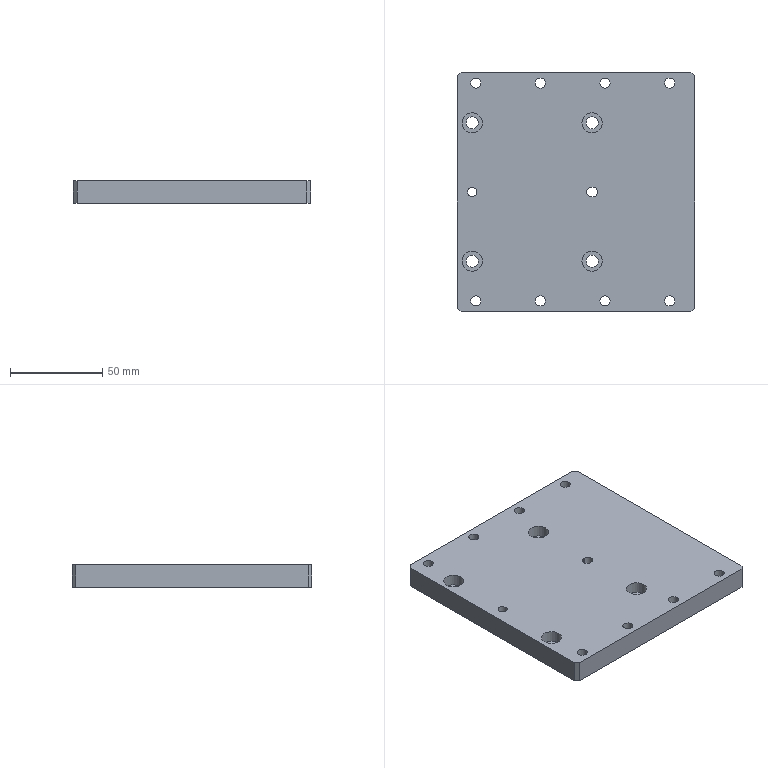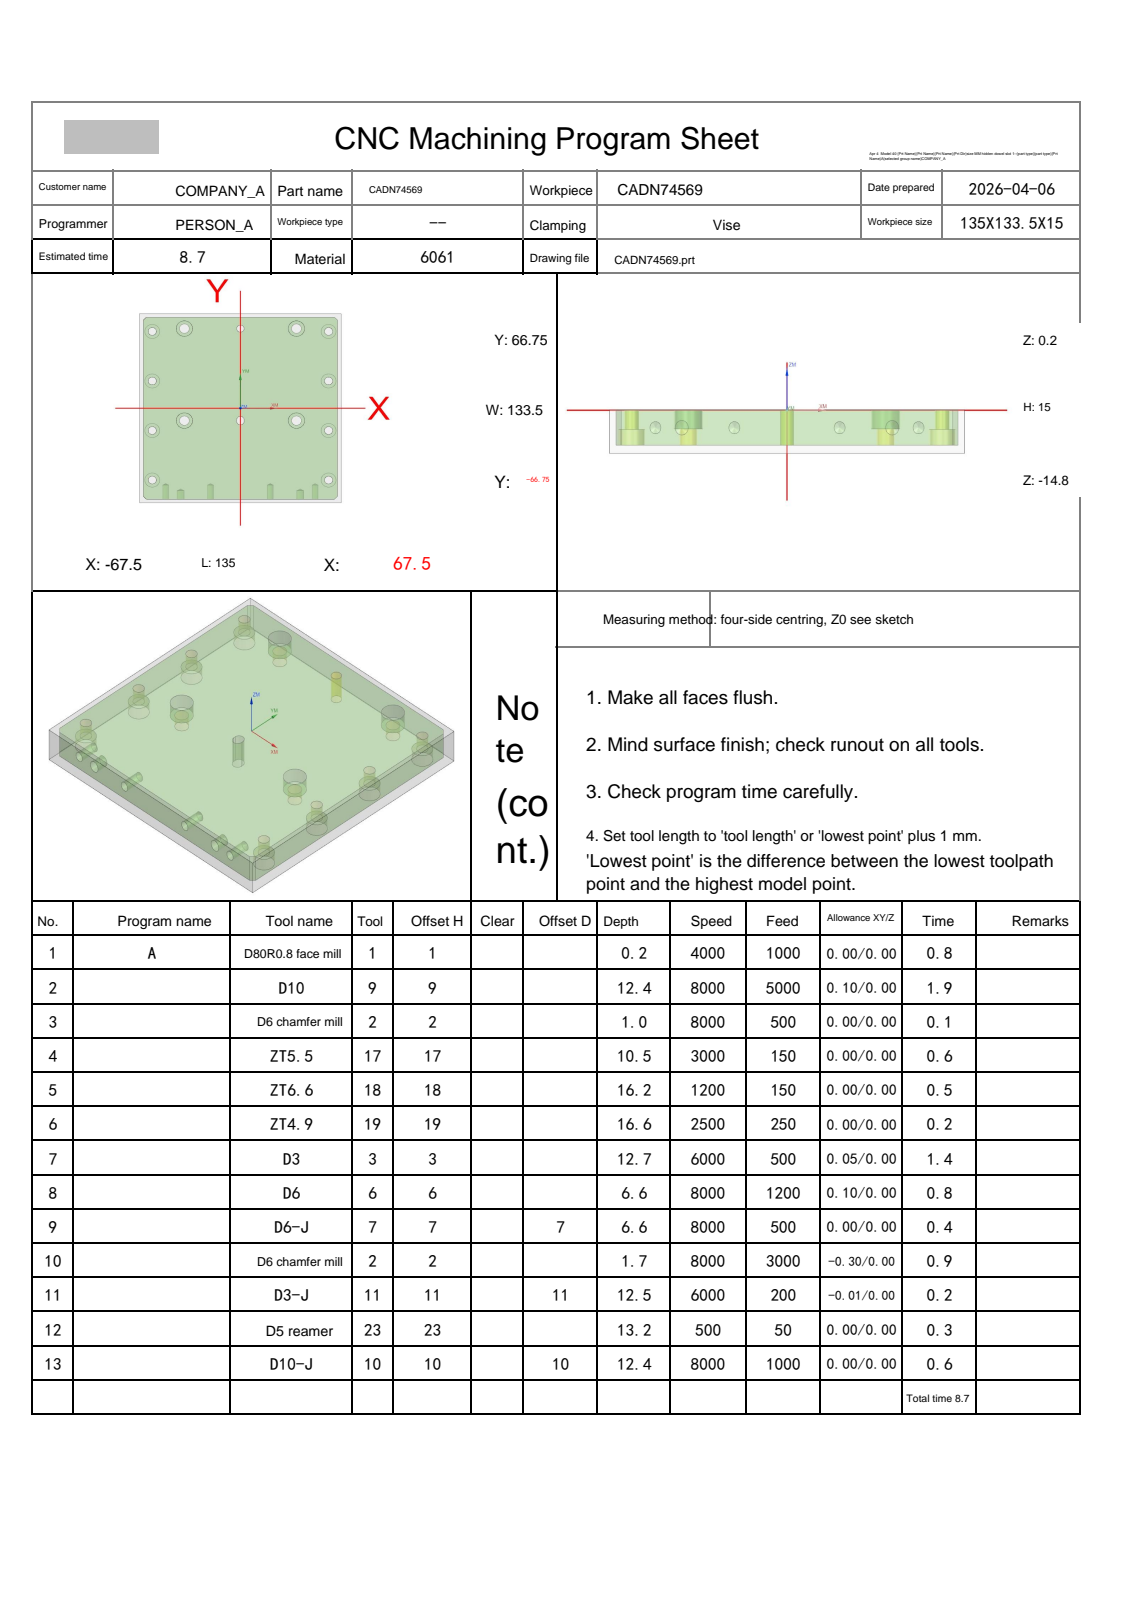NC program | NX | posted by the shop | part box 128.5 x 130 x 12 mm
Whole program, first 1332 of 1585 lines:
%
O0001
(Machine time: 11.02 MIN)
(===Total Tool:12===)
(T1=D80R0.8 face mill D=80.  R=0.8  D-  H01 Z=0.    )
(T9=D10     D=10.  R=0.   D-  H09 Z=-12.2 )
(T2=D6 chamfer mill   D=6.   R=0.   D-  H02 Z=-1.5  )
(T17=ZT5.5  D=5.5  DR_a=118 D-  H17 Z=-10.25)
(T18=ZT6.6  D=6.6  DR_a=118 D-  H18 Z=-15.98)
(T19=ZT4.9  D=4.9  DR_a=120 D-  H19 Z=-16.41)
(T3=D3      D=3.   R=0.   D-  H03 Z=-12.5 )
(T6=D6      D=6.   R=0.   D-  H06 Z=-6.4  )
(T7=D6-J    D=6.   R=0.   D7  H07 Z=-6.4  )
(T11=D3-J   D=3.   R=0.   D11 H11 Z=-12.3 )
(T23=D5 reamer   D=5.   DR_a=180 D-  H23 Z=-13.  )
(T10=D10-J  D=10.  R=0.   D10 H10 Z=-12.2 )
G80 G90 G17 G49 G40
G91 G28 Z0
M01
N1 T01 M06
(D80R0.8 face mill  D=80. R=0.8 H=01 ce=0.00 di=0.00)
G00 G90 G54 X-110. Y52.125 M03 S4000
G43 H01 Z20.
M08
Z2.
G01 Z0.0 F1000.
X-105.
X105.
Y0.0
X-105.
Y-52.125
X105.
X110.
Z2.
G00 Z20.
G91 G28 Z0.0
M05
M09
G91 G28 Z0.0
M01
N2 T09 M06
(D10  D=10. R=0. H=09 ce=0.10 di=0.00)
G00 G90 G54 X0.0 Y69.35 M03 S8000
G43 H09 Z20.
M08
Z.5
G01 X63. Z.408 F5000.
G02 X66.606 Y67.856 Z.402 I0.0 J-5.1
G01 X68.606 Y65.856 Z.398
G02 X70.1 Y62.25 Z.392 I-3.606 J-3.606
G01 Y-62.25 Z.211
G02 X68.606 Y-65.856 Z.205 I-5.1 J0.0
G01 X66.606 Y-67.856 Z.201
G02 X63. Y-69.35 Z.195 I-3.606 J3.606
G01 X-63. Z.011
G02 X-66.606 Y-67.856 Z.005 I0.0 J5.1
G01 X-68.606 Y-65.856 Z.001
G02 X-70.1 Y-62.25 Z-.005 I3.606 J3.606
G01 Y62.25 Z-.186
G02 X-68.606 Y65.856 Z-.192 I5.1 J0.0
G01 X-66.606 Y67.856 Z-.196
G02 X-63. Y69.35 Z-.202 I3.606 J-3.606
G01 X63. Z-.386
G02 X66.606 Y67.856 Z-.391 I0.0 J-5.1
G01 X68.606 Y65.856 Z-.396
G02 X70.1 Y62.25 Z-.401 I-3.606 J-3.606
G01 Y-62.25 Z-.583
G02 X68.606 Y-65.856 Z-.589 I-5.1 J0.0
G01 X66.606 Y-67.856 Z-.593
G02 X63. Y-69.35 Z-.599 I-3.606 J3.606
G01 X-63. Z-.782
G02 X-66.606 Y-67.856 Z-.788 I0.0 J5.1
G01 X-68.606 Y-65.856 Z-.792
G02 X-70.1 Y-62.25 Z-.798 I3.606 J3.606
G01 Y62.25 Z-.98
G02 X-68.606 Y65.856 Z-.986 I5.1 J0.0
G01 X-66.606 Y67.856 Z-.99
G02 X-63. Y69.35 Z-.996 I3.606 J-3.606
G01 X63. Z-1.179
G02 X66.606 Y67.856 Z-1.185 I0.0 J-5.1
G01 X68.606 Y65.856 Z-1.189
G02 X70.1 Y62.25 Z-1.195 I-3.606 J-3.606
G01 Y-62.25 Z-1.377
G02 X68.606 Y-65.856 Z-1.383 I-5.1 J0.0
G01 X66.606 Y-67.856 Z-1.387
G02 X63. Y-69.35 Z-1.393 I-3.606 J3.606
G01 X-63. Z-1.576
G02 X-66.606 Y-67.856 Z-1.582 I0.0 J5.1
G01 X-68.606 Y-65.856 Z-1.586
G02 X-70.1 Y-62.25 Z-1.592 I3.606 J3.606
G01 Y62.25 Z-1.774
G02 X-68.606 Y65.856 Z-1.779 I5.1 J0.0
G01 X-66.606 Y67.856 Z-1.784
G02 X-63. Y69.35 Z-1.789 I3.606 J-3.606
G01 X63. Z-1.973
G02 X66.606 Y67.856 Z-1.979 I0.0 J-5.1
G01 X68.606 Y65.856 Z-1.983
G02 X70.1 Y62.25 Z-1.989 I-3.606 J-3.606
G01 Y-62.25 Z-2.17
G02 X68.606 Y-65.856 Z-2.176 I-5.1 J0.0
G01 X66.606 Y-67.856 Z-2.18
G02 X63. Y-69.35 Z-2.186 I-3.606 J3.606
G01 X-63. Z-2.37
G02 X-66.606 Y-67.856 Z-2.376 I0.0 J5.1
G01 X-68.606 Y-65.856 Z-2.38
G02 X-70.1 Y-62.25 Z-2.386 I3.606 J3.606
G01 Y62.25 Z-2.567
G02 X-68.606 Y65.856 Z-2.573 I5.1 J0.0
G01 X-66.606 Y67.856 Z-2.577
G02 X-63. Y69.35 Z-2.583 I3.606 J-3.606
G01 X63. Z-2.767
G02 X66.606 Y67.856 Z-2.773 I0.0 J-5.1
G01 X68.606 Y65.856 Z-2.777
G02 X70.1 Y62.25 Z-2.783 I-3.606 J-3.606
G01 Y-62.25 Z-2.964
G02 X68.606 Y-65.856 Z-2.97 I-5.1 J0.0
G01 X66.606 Y-67.856 Z-2.974
G02 X63. Y-69.35 Z-2.98 I-3.606 J3.606
G01 X-63. Z-3.164
G02 X-66.606 Y-67.856 Z-3.17 I0.0 J5.1
G01 X-68.606 Y-65.856 Z-3.174
G02 X-70.1 Y-62.25 Z-3.18 I3.606 J3.606
G01 Y62.25 Z-3.361
G02 X-68.606 Y65.856 Z-3.367 I5.1 J0.0
G01 X-66.606 Y67.856 Z-3.371
G02 X-63. Y69.35 Z-3.377 I3.606 J-3.606
G01 X63. Z-3.561
G02 X66.606 Y67.856 Z-3.566 I0.0 J-5.1
G01 X68.606 Y65.856 Z-3.571
G02 X70.1 Y62.25 Z-3.576 I-3.606 J-3.606
G01 Y-62.25 Z-3.758
G02 X68.606 Y-65.856 Z-3.764 I-5.1 J0.0
G01 X66.606 Y-67.856 Z-3.768
G02 X63. Y-69.35 Z-3.774 I-3.606 J3.606
G01 X-63. Z-3.957
G02 X-66.606 Y-67.856 Z-3.963 I0.0 J5.1
G01 X-68.606 Y-65.856 Z-3.967
G02 X-70.1 Y-62.25 Z-3.973 I3.606 J3.606
G01 Y62.25 Z-4.155
G02 X-68.606 Y65.856 Z-4.161 I5.1 J0.0
G01 X-66.606 Y67.856 Z-4.165
G02 X-63. Y69.35 Z-4.171 I3.606 J-3.606
G01 X63. Z-4.354
G02 X66.606 Y67.856 Z-4.36 I0.0 J-5.1
G01 X68.606 Y65.856 Z-4.364
G02 X70.1 Y62.25 Z-4.37 I-3.606 J-3.606
G01 Y-62.25 Z-4.552
G02 X68.606 Y-65.856 Z-4.558 I-5.1 J0.0
G01 X66.606 Y-67.856 Z-4.562
G02 X63. Y-69.35 Z-4.568 I-3.606 J3.606
G01 X-63. Z-4.751
G02 X-66.606 Y-67.856 Z-4.757 I0.0 J5.1
G01 X-68.606 Y-65.856 Z-4.761
G02 X-70.1 Y-62.25 Z-4.767 I3.606 J3.606
G01 Y62.25 Z-4.949
G02 X-68.606 Y65.856 Z-4.954 I5.1 J0.0
G01 X-66.606 Y67.856 Z-4.959
G02 X-63. Y69.35 Z-4.964 I3.606 J-3.606
G01 X63. Z-5.148
G02 X66.606 Y67.856 Z-5.154 I0.0 J-5.1
G01 X68.606 Y65.856 Z-5.158
G02 X70.1 Y62.25 Z-5.164 I-3.606 J-3.606
G01 Y-62.25 Z-5.345
G02 X68.606 Y-65.856 Z-5.351 I-5.1 J0.0
G01 X66.606 Y-67.856 Z-5.355
G02 X63. Y-69.35 Z-5.361 I-3.606 J3.606
G01 X-63. Z-5.545
G02 X-66.606 Y-67.856 Z-5.551 I0.0 J5.1
G01 X-68.606 Y-65.856 Z-5.555
G02 X-70.1 Y-62.25 Z-5.561 I3.606 J3.606
G01 Y62.25 Z-5.742
G02 X-68.606 Y65.856 Z-5.748 I5.1 J0.0
G01 X-66.606 Y67.856 Z-5.752
G02 X-63. Y69.35 Z-5.758 I3.606 J-3.606
G01 X63. Z-5.942
G02 X66.606 Y67.856 Z-5.948 I0.0 J-5.1
G01 X68.606 Y65.856 Z-5.952
G02 X70.1 Y62.25 Z-5.958 I-3.606 J-3.606
G01 Y-62.25 Z-6.139
G02 X68.606 Y-65.856 Z-6.145 I-5.1 J0.0
G01 X66.606 Y-67.856 Z-6.149
G02 X63. Y-69.35 Z-6.155 I-3.606 J3.606
G01 X-63. Z-6.339
G02 X-66.606 Y-67.856 Z-6.345 I0.0 J5.1
G01 X-68.606 Y-65.856 Z-6.349
G02 X-70.1 Y-62.25 Z-6.355 I3.606 J3.606
G01 Y62.25 Z-6.536
G02 X-68.606 Y65.856 Z-6.542 I5.1 J0.0
G01 X-66.606 Y67.856 Z-6.546
G02 X-63. Y69.35 Z-6.552 I3.606 J-3.606
G01 X63. Z-6.736
G02 X66.606 Y67.856 Z-6.741 I0.0 J-5.1
G01 X68.606 Y65.856 Z-6.746
G02 X70.1 Y62.25 Z-6.751 I-3.606 J-3.606
G01 Y-62.25 Z-6.933
G02 X68.606 Y-65.856 Z-6.939 I-5.1 J0.0
G01 X66.606 Y-67.856 Z-6.943
G02 X63. Y-69.35 Z-6.949 I-3.606 J3.606
G01 X-63. Z-7.132
G02 X-66.606 Y-67.856 Z-7.138 I0.0 J5.1
G01 X-68.606 Y-65.856 Z-7.142
G02 X-70.1 Y-62.25 Z-7.148 I3.606 J3.606
G01 Y62.25 Z-7.33
G02 X-68.606 Y65.856 Z-7.336 I5.1 J0.0
G01 X-66.606 Y67.856 Z-7.34
G02 X-63. Y69.35 Z-7.346 I3.606 J-3.606
G01 X63. Z-7.529
G02 X66.606 Y67.856 Z-7.535 I0.0 J-5.1
G01 X68.606 Y65.856 Z-7.539
G02 X70.1 Y62.25 Z-7.545 I-3.606 J-3.606
G01 Y-62.25 Z-7.727
G02 X68.606 Y-65.856 Z-7.733 I-5.1 J0.0
G01 X66.606 Y-67.856 Z-7.737
G02 X63. Y-69.35 Z-7.743 I-3.606 J3.606
G01 X-63. Z-7.926
G02 X-66.606 Y-67.856 Z-7.932 I0.0 J5.1
G01 X-68.606 Y-65.856 Z-7.936
G02 X-70.1 Y-62.25 Z-7.942 I3.606 J3.606
G01 Y62.25 Z-8.124
G02 X-68.606 Y65.856 Z-8.129 I5.1 J0.0
G01 X-66.606 Y67.856 Z-8.134
G02 X-63. Y69.35 Z-8.139 I3.606 J-3.606
G01 X63. Z-8.323
G02 X66.606 Y67.856 Z-8.329 I0.0 J-5.1
G01 X68.606 Y65.856 Z-8.333
G02 X70.1 Y62.25 Z-8.339 I-3.606 J-3.606
G01 Y-62.25 Z-8.52
G02 X68.606 Y-65.856 Z-8.526 I-5.1 J0.0
G01 X66.606 Y-67.856 Z-8.53
G02 X63. Y-69.35 Z-8.536 I-3.606 J3.606
G01 X-63. Z-8.72
G02 X-66.606 Y-67.856 Z-8.726 I0.0 J5.1
G01 X-68.606 Y-65.856 Z-8.73
G02 X-70.1 Y-62.25 Z-8.736 I3.606 J3.606
G01 Y62.25 Z-8.917
G02 X-68.606 Y65.856 Z-8.923 I5.1 J0.0
G01 X-66.606 Y67.856 Z-8.927
G02 X-63. Y69.35 Z-8.933 I3.606 J-3.606
G01 X63. Z-9.117
G02 X66.606 Y67.856 Z-9.123 I0.0 J-5.1
G01 X68.606 Y65.856 Z-9.127
G02 X70.1 Y62.25 Z-9.133 I-3.606 J-3.606
G01 Y-62.25 Z-9.314
G02 X68.606 Y-65.856 Z-9.32 I-5.1 J0.0
G01 X66.606 Y-67.856 Z-9.324
G02 X63. Y-69.35 Z-9.33 I-3.606 J3.606
G01 X-63. Z-9.514
G02 X-66.606 Y-67.856 Z-9.52 I0.0 J5.1
G01 X-68.606 Y-65.856 Z-9.524
G02 X-70.1 Y-62.25 Z-9.53 I3.606 J3.606
G01 Y62.25 Z-9.711
G02 X-68.606 Y65.856 Z-9.717 I5.1 J0.0
G01 X-66.606 Y67.856 Z-9.721
G02 X-63. Y69.35 Z-9.727 I3.606 J-3.606
G01 X63. Z-9.911
G02 X66.606 Y67.856 Z-9.916 I0.0 J-5.1
G01 X68.606 Y65.856 Z-9.921
G02 X70.1 Y62.25 Z-9.926 I-3.606 J-3.606
G01 Y-62.25 Z-10.108
G02 X68.606 Y-65.856 Z-10.114 I-5.1 J0.0
G01 X66.606 Y-67.856 Z-10.118
G02 X63. Y-69.35 Z-10.124 I-3.606 J3.606
G01 X-63. Z-10.307
G02 X-66.606 Y-67.856 Z-10.313 I0.0 J5.1
G01 X-68.606 Y-65.856 Z-10.317
G02 X-70.1 Y-62.25 Z-10.323 I3.606 J3.606
G01 Y62.25 Z-10.505
G02 X-68.606 Y65.856 Z-10.511 I5.1 J0.0
G01 X-66.606 Y67.856 Z-10.515
G02 X-63. Y69.35 Z-10.521 I3.606 J-3.606
G01 X63. Z-10.704
G02 X66.606 Y67.856 Z-10.71 I0.0 J-5.1
G01 X68.606 Y65.856 Z-10.714
G02 X70.1 Y62.25 Z-10.72 I-3.606 J-3.606
G01 Y-62.25 Z-10.902
G02 X68.606 Y-65.856 Z-10.908 I-5.1 J0.0
G01 X66.606 Y-67.856 Z-10.912
G02 X63. Y-69.35 Z-10.918 I-3.606 J3.606
G01 X-63. Z-11.101
G02 X-66.606 Y-67.856 Z-11.107 I0.0 J5.1
G01 X-68.606 Y-65.856 Z-11.111
G02 X-70.1 Y-62.25 Z-11.117 I3.606 J3.606
G01 Y62.25 Z-11.299
G02 X-68.606 Y65.856 Z-11.304 I5.1 J0.0
G01 X-66.606 Y67.856 Z-11.309
G02 X-63. Y69.35 Z-11.314 I3.606 J-3.606
G01 X63. Z-11.498
G02 X66.606 Y67.856 Z-11.504 I0.0 J-5.1
G01 X68.606 Y65.856 Z-11.508
G02 X70.1 Y62.25 Z-11.514 I-3.606 J-3.606
G01 Y-62.25 Z-11.695
G02 X68.606 Y-65.856 Z-11.701 I-5.1 J0.0
G01 X66.606 Y-67.856 Z-11.705
G02 X63. Y-69.35 Z-11.711 I-3.606 J3.606
G01 X-63. Z-11.895
G02 X-66.606 Y-67.856 Z-11.901 I0.0 J5.1
G01 X-68.606 Y-65.856 Z-11.905
G02 X-70.1 Y-62.25 Z-11.911 I3.606 J3.606
G01 Y62.25 Z-12.092
G02 X-68.606 Y65.856 Z-12.098 I5.1 J0.0
G01 X-66.606 Y67.856 Z-12.102
G02 X-63. Y69.35 Z-12.108 I3.606 J-3.606
G01 X0.0 Z-12.2
X63.
G02 X66.606 Y67.856 I0.0 J-5.1
G01 X68.606 Y65.856
G02 X70.1 Y62.25 I-3.606 J-3.606
G01 Y-62.25
G02 X68.606 Y-65.856 I-5.1 J0.0
G01 X66.606 Y-67.856
G02 X63. Y-69.35 I-3.606 J3.606
G01 X-63.
G02 X-66.606 Y-67.856 I0.0 J5.1
G01 X-68.606 Y-65.856
G02 X-70.1 Y-62.25 I3.606 J3.606
G01 Y62.25
G02 X-68.606 Y65.856 I5.1 J0.0
G01 X-66.606 Y67.856
G02 X-63. Y69.35 I3.606 J-3.606
G01 X0.0
X.5
Z-11.2
G00 Z20.
G91 G28 Z0.0
M05
M09
G91 G28 Z0.0
M01
N3 T02 M06
(D6 chamfer mill  D=6. R=0. H=02 ce=0.00 di=0.00)
G00 G90 G54 X59. Y-50.75 M03 S8000
G43 H02 Z20.
M08
G98 G81 X59. Y-50.75 Z-.8 R1. F500.
Y-15.75
X37.5 Y-8.75
X59. Y19.25
Y54.25
X37.5 Y56.25
X0.0
X-37.5
X-59. Y54.25
Y19.25
X-37.5 Y-8.75
X-59. Y-15.75
Y-50.75
X0.0 Y-8.25
G80
G00 Z20.
G91 G28 Z0.0
M05
M09
G91 G28 Z0.0
M01
N4 T17 M06
(ZT5.5 D=5.5 DR_a=118 H=17)
G00 G90 G54 X59. Y-50.75 M03 S3000
G43 H17 Z20.
M08
G98 G83 X59. Y-50.75 Z-10.252 R1. F150. Q3.
Y-15.75
Y19.25
Y54.25
X-59.
Y19.25
Y-15.75
Y-50.75
G80
G00 Z20.
G91 G28 Z0.0
M05
M09
G91 G28 Z0.0
M01
N5 T18 M06
(ZT6.6 D=6.6 DR_a=118 H=18)
G00 G90 G54 X-37.5 Y-8.75 M03 S1200
G43 H18 Z20.
M08
G98 G83 X-37.5 Y-8.75 Z-15.983 R1. F150. Q2.
Y56.25
X37.5
Y-8.75
G80
G00 Z20.
G91 G28 Z0.0
M05
M09
G91 G28 Z0.0
M01
N6 T19 M06
(ZT4.9 D=4.9 DR_a=120 H=19)
G00 G90 G54 X0.0 Y56.25 M03 S2500
G43 H19 Z20.
M08
G98 G83 X0.0 Y56.25 Z-16.415 R1. F250. Q2.
Y-8.25
G80
G00 Z20.
G91 G28 Z0.0
M05
M09
G91 G28 Z0.0
M01
N7 T03 M06
(D3  D=3. R=0. H=03 ce=0.05 di=0.00)
G00 G90 G54 X.95 Y-8.75 M03 S6000
G43 H03 Z20.
M08
Z.5
G01 Y-8.25 Z.491 F500.
G03 X0.0 Y-7.3 Z.463 I-.95 J0.0
X-.95 Y-8.25 Z.435 I0.0 J-.95
G01 Y-9.25 Z.416
G03 X0.0 Y-10.2 Z.388 I.95 J0.0
X.95 Y-9.25 Z.36 I0.0 J.95
G01 Y-8.25 Z.341
G03 X0.0 Y-7.3 Z.313 I-.95 J0.0
X-.95 Y-8.25 Z.285 I0.0 J-.95
G01 Y-9.25 Z.266
G03 X0.0 Y-10.2 Z.239 I.95 J0.0
X.95 Y-9.25 Z.211 I0.0 J.95
G01 Y-8.25 Z.192
G03 X0.0 Y-7.3 Z.164 I-.95 J0.0
X-.95 Y-8.25 Z.136 I0.0 J-.95
G01 Y-9.25 Z.117
G03 X0.0 Y-10.2 Z.089 I.95 J0.0
X.95 Y-9.25 Z.061 I0.0 J.95
G01 Y-8.25 Z.042
G03 X0.0 Y-7.3 Z.014 I-.95 J0.0
X-.95 Y-8.25 Z-.014 I0.0 J-.95
G01 Y-9.25 Z-.032
G03 X0.0 Y-10.2 Z-.06 I.95 J0.0
X.95 Y-9.25 Z-.088 I0.0 J.95
G01 Y-8.25 Z-.107
G03 X0.0 Y-7.3 Z-.135 I-.95 J0.0
X-.95 Y-8.25 Z-.163 I0.0 J-.95
G01 Y-9.25 Z-.182
G03 X0.0 Y-10.2 Z-.21 I.95 J0.0
X.95 Y-9.25 Z-.238 I0.0 J.95
G01 Y-8.25 Z-.257
G03 X0.0 Y-7.3 Z-.284 I-.95 J0.0
X-.95 Y-8.25 Z-.312 I0.0 J-.95
G01 Y-9.25 Z-.331
G03 X0.0 Y-10.2 Z-.359 I.95 J0.0
X.95 Y-9.25 Z-.387 I0.0 J.95
G01 Y-8.25 Z-.406
G03 X0.0 Y-7.3 Z-.434 I-.95 J0.0
X-.95 Y-8.25 Z-.462 I0.0 J-.95
G01 Y-9.25 Z-.481
G03 X0.0 Y-10.2 Z-.509 I.95 J0.0
X.95 Y-9.25 Z-.537 I0.0 J.95
G01 Y-8.25 Z-.555
G03 X0.0 Y-7.3 Z-.583 I-.95 J0.0
X-.95 Y-8.25 Z-.611 I0.0 J-.95
G01 Y-9.25 Z-.63
G03 X0.0 Y-10.2 Z-.658 I.95 J0.0
X.95 Y-9.25 Z-.686 I0.0 J.95
G01 Y-8.25 Z-.705
G03 X0.0 Y-7.3 Z-.733 I-.95 J0.0
X-.95 Y-8.25 Z-.761 I0.0 J-.95
G01 Y-9.25 Z-.779
G03 X0.0 Y-10.2 Z-.807 I.95 J0.0
X.95 Y-9.25 Z-.835 I0.0 J.95
G01 Y-8.25 Z-.854
G03 X0.0 Y-7.3 Z-.882 I-.95 J0.0
X-.95 Y-8.25 Z-.91 I0.0 J-.95
G01 Y-9.25 Z-.929
G03 X0.0 Y-10.2 Z-.957 I.95 J0.0
X.95 Y-9.25 Z-.985 I0.0 J.95
G01 Y-8.25 Z-1.004
G03 X0.0 Y-7.3 Z-1.032 I-.95 J0.0
X-.95 Y-8.25 Z-1.06 I0.0 J-.95
G01 Y-9.25 Z-1.078
G03 X0.0 Y-10.2 Z-1.106 I.95 J0.0
X.95 Y-9.25 Z-1.134 I0.0 J.95
G01 Y-8.25 Z-1.153
G03 X0.0 Y-7.3 Z-1.181 I-.95 J0.0
X-.95 Y-8.25 Z-1.209 I0.0 J-.95
G01 Y-9.25 Z-1.228
G03 X0.0 Y-10.2 Z-1.256 I.95 J0.0
X.95 Y-9.25 Z-1.284 I0.0 J.95
G01 Y-8.25 Z-1.302
G03 X0.0 Y-7.3 Z-1.33 I-.95 J0.0
X-.95 Y-8.25 Z-1.358 I0.0 J-.95
G01 Y-9.25 Z-1.377
G03 X0.0 Y-10.2 Z-1.405 I.95 J0.0
X.95 Y-9.25 Z-1.433 I0.0 J.95
G01 Y-8.25 Z-1.452
G03 X0.0 Y-7.3 Z-1.48 I-.95 J0.0
X-.95 Y-8.25 Z-1.508 I0.0 J-.95
G01 Y-9.25 Z-1.527
G03 X0.0 Y-10.2 Z-1.555 I.95 J0.0
X.95 Y-9.25 Z-1.583 I0.0 J.95
G01 Y-8.25 Z-1.601
G03 X0.0 Y-7.3 Z-1.629 I-.95 J0.0
X-.95 Y-8.25 Z-1.657 I0.0 J-.95
G01 Y-9.25 Z-1.676
G03 X0.0 Y-10.2 Z-1.704 I.95 J0.0
X.95 Y-9.25 Z-1.732 I0.0 J.95
G01 Y-8.25 Z-1.751
G03 X0.0 Y-7.3 Z-1.779 I-.95 J0.0
X-.95 Y-8.25 Z-1.807 I0.0 J-.95
G01 Y-9.25 Z-1.825
G03 X0.0 Y-10.2 Z-1.853 I.95 J0.0
X.95 Y-9.25 Z-1.881 I0.0 J.95
G01 Y-8.25 Z-1.9
G03 X0.0 Y-7.3 Z-1.928 I-.95 J0.0
X-.95 Y-8.25 Z-1.956 I0.0 J-.95
G01 Y-9.25 Z-1.975
G03 X0.0 Y-10.2 Z-2.003 I.95 J0.0
X.95 Y-9.25 Z-2.031 I0.0 J.95
G01 Y-8.25 Z-2.05
G03 X0.0 Y-7.3 Z-2.078 I-.95 J0.0
X-.95 Y-8.25 Z-2.106 I0.0 J-.95
G01 Y-9.25 Z-2.124
G03 X0.0 Y-10.2 Z-2.152 I.95 J0.0
X.95 Y-9.25 Z-2.18 I0.0 J.95
G01 Y-8.25 Z-2.199
G03 X0.0 Y-7.3 Z-2.227 I-.95 J0.0
X-.95 Y-8.25 Z-2.255 I0.0 J-.95
G01 Y-9.25 Z-2.274
G03 X0.0 Y-10.2 Z-2.302 I.95 J0.0
X.95 Y-9.25 Z-2.33 I0.0 J.95
G01 Y-8.25 Z-2.348
G03 X0.0 Y-7.3 Z-2.376 I-.95 J0.0
X-.95 Y-8.25 Z-2.404 I0.0 J-.95
G01 Y-9.25 Z-2.423
G03 X0.0 Y-10.2 Z-2.451 I.95 J0.0
X.95 Y-9.25 Z-2.479 I0.0 J.95
G01 Y-8.25 Z-2.498
G03 X0.0 Y-7.3 Z-2.526 I-.95 J0.0
X-.95 Y-8.25 Z-2.554 I0.0 J-.95
G01 Y-9.25 Z-2.573
G03 X0.0 Y-10.2 Z-2.601 I.95 J0.0
X.95 Y-9.25 Z-2.629 I0.0 J.95
G01 Y-8.25 Z-2.647
G03 X0.0 Y-7.3 Z-2.675 I-.95 J0.0
X-.95 Y-8.25 Z-2.703 I0.0 J-.95
G01 Y-9.25 Z-2.722
G03 X0.0 Y-10.2 Z-2.75 I.95 J0.0
X.95 Y-9.25 Z-2.778 I0.0 J.95
G01 Y-8.25 Z-2.797
G03 X0.0 Y-7.3 Z-2.825 I-.95 J0.0
X-.95 Y-8.25 Z-2.853 I0.0 J-.95
G01 Y-9.25 Z-2.871
G03 X0.0 Y-10.2 Z-2.899 I.95 J0.0
X.95 Y-9.25 Z-2.927 I0.0 J.95
G01 Y-8.25 Z-2.946
G03 X0.0 Y-7.3 Z-2.974 I-.95 J0.0
X-.95 Y-8.25 Z-3.002 I0.0 J-.95
G01 Y-9.25 Z-3.021
G03 X0.0 Y-10.2 Z-3.049 I.95 J0.0
X.95 Y-9.25 Z-3.077 I0.0 J.95
G01 Y-8.25 Z-3.096
G03 X0.0 Y-7.3 Z-3.124 I-.95 J0.0
X-.95 Y-8.25 Z-3.152 I0.0 J-.95
G01 Y-9.25 Z-3.17
G03 X0.0 Y-10.2 Z-3.198 I.95 J0.0
X.95 Y-9.25 Z-3.226 I0.0 J.95
G01 Y-8.25 Z-3.245
G03 X0.0 Y-7.3 Z-3.273 I-.95 J0.0
X-.95 Y-8.25 Z-3.301 I0.0 J-.95
G01 Y-9.25 Z-3.32
G03 X0.0 Y-10.2 Z-3.348 I.95 J0.0
X.95 Y-9.25 Z-3.376 I0.0 J.95
G01 Y-8.25 Z-3.394
G03 X0.0 Y-7.3 Z-3.422 I-.95 J0.0
X-.95 Y-8.25 Z-3.45 I0.0 J-.95
G01 Y-9.25 Z-3.469
G03 X0.0 Y-10.2 Z-3.497 I.95 J0.0
X.95 Y-9.25 Z-3.525 I0.0 J.95
G01 Y-8.25 Z-3.544
G03 X0.0 Y-7.3 Z-3.572 I-.95 J0.0
X-.95 Y-8.25 Z-3.6 I0.0 J-.95
G01 Y-9.25 Z-3.619
G03 X0.0 Y-10.2 Z-3.647 I.95 J0.0
X.95 Y-9.25 Z-3.675 I0.0 J.95
G01 Y-8.25 Z-3.693
G03 X0.0 Y-7.3 Z-3.721 I-.95 J0.0
X-.95 Y-8.25 Z-3.749 I0.0 J-.95
G01 Y-9.25 Z-3.768
G03 X0.0 Y-10.2 Z-3.796 I.95 J0.0
X.95 Y-9.25 Z-3.824 I0.0 J.95
G01 Y-8.25 Z-3.843
G03 X0.0 Y-7.3 Z-3.871 I-.95 J0.0
X-.95 Y-8.25 Z-3.899 I0.0 J-.95
G01 Y-9.25 Z-3.917
G03 X0.0 Y-10.2 Z-3.945 I.95 J0.0
X.95 Y-9.25 Z-3.973 I0.0 J.95
G01 Y-8.25 Z-3.992
G03 X0.0 Y-7.3 Z-4.02 I-.95 J0.0
X-.95 Y-8.25 Z-4.048 I0.0 J-.95
G01 Y-9.25 Z-4.067
G03 X0.0 Y-10.2 Z-4.095 I.95 J0.0
X.95 Y-9.25 Z-4.123 I0.0 J.95
G01 Y-8.25 Z-4.142
G03 X0.0 Y-7.3 Z-4.17 I-.95 J0.0
X-.95 Y-8.25 Z-4.198 I0.0 J-.95
G01 Y-9.25 Z-4.216
G03 X0.0 Y-10.2 Z-4.244 I.95 J0.0
X.95 Y-9.25 Z-4.272 I0.0 J.95
G01 Y-8.25 Z-4.291
G03 X0.0 Y-7.3 Z-4.319 I-.95 J0.0
X-.95 Y-8.25 Z-4.347 I0.0 J-.95
G01 Y-9.25 Z-4.366
G03 X0.0 Y-10.2 Z-4.394 I.95 J0.0
X.95 Y-9.25 Z-4.422 I0.0 J.95
G01 Y-8.25 Z-4.44
G03 X0.0 Y-7.3 Z-4.468 I-.95 J0.0
X-.95 Y-8.25 Z-4.496 I0.0 J-.95
G01 Y-9.25 Z-4.515
G03 X0.0 Y-10.2 Z-4.543 I.95 J0.0
X.95 Y-9.25 Z-4.571 I0.0 J.95
G01 Y-8.25 Z-4.59
G03 X0.0 Y-7.3 Z-4.618 I-.95 J0.0
X-.95 Y-8.25 Z-4.646 I0.0 J-.95
G01 Y-9.25 Z-4.665
G03 X0.0 Y-10.2 Z-4.693 I.95 J0.0
X.95 Y-9.25 Z-4.721 I0.0 J.95
G01 Y-8.25 Z-4.739
G03 X0.0 Y-7.3 Z-4.767 I-.95 J0.0
X-.95 Y-8.25 Z-4.795 I0.0 J-.95
G01 Y-9.25 Z-4.814
G03 X0.0 Y-10.2 Z-4.842 I.95 J0.0
X.95 Y-9.25 Z-4.87 I0.0 J.95
G01 Y-8.25 Z-4.889
G03 X0.0 Y-7.3 Z-4.917 I-.95 J0.0
X-.95 Y-8.25 Z-4.945 I0.0 J-.95
G01 Y-9.25 Z-4.963
G03 X0.0 Y-10.2 Z-4.991 I.95 J0.0
X.95 Y-9.25 Z-5.019 I0.0 J.95
G01 Y-8.25 Z-5.038
G03 X0.0 Y-7.3 Z-5.066 I-.95 J0.0
X-.95 Y-8.25 Z-5.094 I0.0 J-.95
G01 Y-9.25 Z-5.113
G03 X0.0 Y-10.2 Z-5.141 I.95 J0.0
X.95 Y-9.25 Z-5.169 I0.0 J.95
G01 Y-8.25 Z-5.188
G03 X0.0 Y-7.3 Z-5.216 I-.95 J0.0
X-.95 Y-8.25 Z-5.243 I0.0 J-.95
G01 Y-9.25 Z-5.262
G03 X0.0 Y-10.2 Z-5.29 I.95 J0.0
X.95 Y-9.25 Z-5.318 I0.0 J.95
G01 Y-8.25 Z-5.337
G03 X0.0 Y-7.3 Z-5.365 I-.95 J0.0
X-.95 Y-8.25 Z-5.393 I0.0 J-.95
G01 Y-9.25 Z-5.412
G03 X0.0 Y-10.2 Z-5.44 I.95 J0.0
X.95 Y-9.25 Z-5.468 I0.0 J.95
G01 Y-8.25 Z-5.486
G03 X0.0 Y-7.3 Z-5.514 I-.95 J0.0
X-.95 Y-8.25 Z-5.542 I0.0 J-.95
G01 Y-9.25 Z-5.561
G03 X0.0 Y-10.2 Z-5.589 I.95 J0.0
X.95 Y-9.25 Z-5.617 I0.0 J.95
G01 Y-8.25 Z-5.636
G03 X0.0 Y-7.3 Z-5.664 I-.95 J0.0
X-.95 Y-8.25 Z-5.692 I0.0 J-.95
G01 Y-9.25 Z-5.711
G03 X0.0 Y-10.2 Z-5.739 I.95 J0.0
X.95 Y-9.25 Z-5.766 I0.0 J.95
G01 Y-8.25 Z-5.785
G03 X0.0 Y-7.3 Z-5.813 I-.95 J0.0
X-.95 Y-8.25 Z-5.841 I0.0 J-.95
G01 Y-9.25 Z-5.86
G03 X0.0 Y-10.2 Z-5.888 I.95 J0.0
X.95 Y-9.25 Z-5.916 I0.0 J.95
G01 Y-8.25 Z-5.935
G03 X0.0 Y-7.3 Z-5.963 I-.95 J0.0
X-.95 Y-8.25 Z-5.991 I0.0 J-.95
G01 Y-9.25 Z-6.009
G03 X0.0 Y-10.2 Z-6.037 I.95 J0.0
X.95 Y-9.25 Z-6.065 I0.0 J.95
G01 Y-8.25 Z-6.084
G03 X0.0 Y-7.3 Z-6.112 I-.95 J0.0
X-.95 Y-8.25 Z-6.14 I0.0 J-.95
G01 Y-9.25 Z-6.159
G03 X0.0 Y-10.2 Z-6.187 I.95 J0.0
X.95 Y-9.25 Z-6.215 I0.0 J.95
G01 Y-8.25 Z-6.234
G03 X0.0 Y-7.3 Z-6.261 I-.95 J0.0
X-.95 Y-8.25 Z-6.289 I0.0 J-.95
G01 Y-9.25 Z-6.308
G03 X0.0 Y-10.2 Z-6.336 I.95 J0.0
X.95 Y-9.25 Z-6.364 I0.0 J.95
G01 Y-8.25 Z-6.383
G03 X0.0 Y-7.3 Z-6.411 I-.95 J0.0
X-.95 Y-8.25 Z-6.439 I0.0 J-.95
G01 Y-9.25 Z-6.458
G03 X0.0 Y-10.2 Z-6.486 I.95 J0.0
X.95 Y-9.25 Z-6.514 I0.0 J.95
G01 Y-8.25 Z-6.532
G03 X0.0 Y-7.3 Z-6.56 I-.95 J0.0
X-.95 Y-8.25 Z-6.588 I0.0 J-.95
G01 Y-9.25 Z-6.607
G03 X0.0 Y-10.2 Z-6.635 I.95 J0.0
X.95 Y-9.25 Z-6.663 I0.0 J.95
G01 Y-8.25 Z-6.682
G03 X0.0 Y-7.3 Z-6.71 I-.95 J0.0
X-.95 Y-8.25 Z-6.738 I0.0 J-.95
G01 Y-9.25 Z-6.757
G03 X0.0 Y-10.2 Z-6.784 I.95 J0.0
X.95 Y-9.25 Z-6.812 I0.0 J.95
G01 Y-8.25 Z-6.831
G03 X0.0 Y-7.3 Z-6.859 I-.95 J0.0
X-.95 Y-8.25 Z-6.887 I0.0 J-.95
G01 Y-9.25 Z-6.906
G03 X0.0 Y-10.2 Z-6.934 I.95 J0.0
X.95 Y-9.25 Z-6.962 I0.0 J.95
G01 Y-8.25 Z-6.981
G03 X0.0 Y-7.3 Z-7.009 I-.95 J0.0
X-.95 Y-8.25 Z-7.037 I0.0 J-.95
G01 Y-9.25 Z-7.055
G03 X0.0 Y-10.2 Z-7.083 I.95 J0.0
X.95 Y-9.25 Z-7.111 I0.0 J.95
G01 Y-8.25 Z-7.13
G03 X0.0 Y-7.3 Z-7.158 I-.95 J0.0
X-.95 Y-8.25 Z-7.186 I0.0 J-.95
G01 Y-9.25 Z-7.205
G03 X0.0 Y-10.2 Z-7.233 I.95 J0.0
X.95 Y-9.25 Z-7.261 I0.0 J.95
G01 Y-8.25 Z-7.279
G03 X0.0 Y-7.3 Z-7.307 I-.95 J0.0
X-.95 Y-8.25 Z-7.335 I0.0 J-.95
G01 Y-9.25 Z-7.354
G03 X0.0 Y-10.2 Z-7.382 I.95 J0.0
X.95 Y-9.25 Z-7.41 I0.0 J.95
G01 Y-8.25 Z-7.429
G03 X0.0 Y-7.3 Z-7.457 I-.95 J0.0
X-.95 Y-8.25 Z-7.485 I0.0 J-.95
G01 Y-9.25 Z-7.504
G03 X0.0 Y-10.2 Z-7.532 I.95 J0.0
X.95 Y-9.25 Z-7.56 I0.0 J.95
G01 Y-8.25 Z-7.578
G03 X0.0 Y-7.3 Z-7.606 I-.95 J0.0
X-.95 Y-8.25 Z-7.634 I0.0 J-.95
G01 Y-9.25 Z-7.653
G03 X0.0 Y-10.2 Z-7.681 I.95 J0.0
X.95 Y-9.25 Z-7.709 I0.0 J.95
G01 Y-8.25 Z-7.728
G03 X0.0 Y-7.3 Z-7.756 I-.95 J0.0
X-.95 Y-8.25 Z-7.784 I0.0 J-.95
G01 Y-9.25 Z-7.802
G03 X0.0 Y-10.2 Z-7.83 I.95 J0.0
X.95 Y-9.25 Z-7.858 I0.0 J.95
G01 Y-8.25 Z-7.877
G03 X0.0 Y-7.3 Z-7.905 I-.95 J0.0
X-.95 Y-8.25 Z-7.933 I0.0 J-.95
G01 Y-9.25 Z-7.952
G03 X0.0 Y-10.2 Z-7.98 I.95 J0.0
X.95 Y-9.25 Z-8.008 I0.0 J.95
G01 Y-8.25 Z-8.027
G03 X0.0 Y-7.3 Z-8.055 I-.95 J0.0
X-.95 Y-8.25 Z-8.083 I0.0 J-.95
G01 Y-9.25 Z-8.101
G03 X0.0 Y-10.2 Z-8.129 I.95 J0.0
X.95 Y-9.25 Z-8.157 I0.0 J.95
G01 Y-8.25 Z-8.176
G03 X0.0 Y-7.3 Z-8.204 I-.95 J0.0
X-.95 Y-8.25 Z-8.232 I0.0 J-.95
G01 Y-9.25 Z-8.251
G03 X0.0 Y-10.2 Z-8.279 I.95 J0.0
X.95 Y-9.25 Z-8.307 I0.0 J.95
G01 Y-8.25 Z-8.325
G03 X0.0 Y-7.3 Z-8.353 I-.95 J0.0
X-.95 Y-8.25 Z-8.381 I0.0 J-.95
G01 Y-9.25 Z-8.4
G03 X0.0 Y-10.2 Z-8.428 I.95 J0.0
X.95 Y-9.25 Z-8.456 I0.0 J.95
G01 Y-8.25 Z-8.475
G03 X0.0 Y-7.3 Z-8.503 I-.95 J0.0
X-.95 Y-8.25 Z-8.531 I0.0 J-.95
G01 Y-9.25 Z-8.55
G03 X0.0 Y-10.2 Z-8.578 I.95 J0.0
X.95 Y-9.25 Z-8.606 I0.0 J.95
G01 Y-8.25 Z-8.624
G03 X0.0 Y-7.3 Z-8.652 I-.95 J0.0
X-.95 Y-8.25 Z-8.68 I0.0 J-.95
G01 Y-9.25 Z-8.699
G03 X0.0 Y-10.2 Z-8.727 I.95 J0.0
X.95 Y-9.25 Z-8.755 I0.0 J.95
G01 Y-8.25 Z-8.774
G03 X0.0 Y-7.3 Z-8.802 I-.95 J0.0
X-.95 Y-8.25 Z-8.83 I0.0 J-.95
G01 Y-9.25 Z-8.848
G03 X0.0 Y-10.2 Z-8.876 I.95 J0.0
X.95 Y-9.25 Z-8.904 I0.0 J.95
G01 Y-8.25 Z-8.923
G03 X0.0 Y-7.3 Z-8.951 I-.95 J0.0
X-.95 Y-8.25 Z-8.979 I0.0 J-.95
G01 Y-9.25 Z-8.998
G03 X0.0 Y-10.2 Z-9.026 I.95 J0.0
X.95 Y-9.25 Z-9.054 I0.0 J.95
G01 Y-8.25 Z-9.073
G03 X0.0 Y-7.3 Z-9.101 I-.95 J0.0
X-.95 Y-8.25 Z-9.129 I0.0 J-.95
G01 Y-9.25 Z-9.147
G03 X0.0 Y-10.2 Z-9.175 I.95 J0.0
X.95 Y-9.25 Z-9.203 I0.0 J.95
G01 Y-8.25 Z-9.222
G03 X0.0 Y-7.3 Z-9.25 I-.95 J0.0
X-.95 Y-8.25 Z-9.278 I0.0 J-.95
G01 Y-9.25 Z-9.297
G03 X0.0 Y-10.2 Z-9.325 I.95 J0.0
X.95 Y-9.25 Z-9.353 I0.0 J.95
G01 Y-8.25 Z-9.371
G03 X0.0 Y-7.3 Z-9.399 I-.95 J0.0
X-.95 Y-8.25 Z-9.427 I0.0 J-.95
G01 Y-9.25 Z-9.446
G03 X0.0 Y-10.2 Z-9.474 I.95 J0.0
X.95 Y-9.25 Z-9.502 I0.0 J.95
G01 Y-8.25 Z-9.521
G03 X0.0 Y-7.3 Z-9.549 I-.95 J0.0
X-.95 Y-8.25 Z-9.577 I0.0 J-.95
G01 Y-9.25 Z-9.596
G03 X0.0 Y-10.2 Z-9.624 I.95 J0.0
X.95 Y-9.25 Z-9.652 I0.0 J.95
G01 Y-8.25 Z-9.67
G03 X0.0 Y-7.3 Z-9.698 I-.95 J0.0
X-.95 Y-8.25 Z-9.726 I0.0 J-.95
G01 Y-9.25 Z-9.745
G03 X0.0 Y-10.2 Z-9.773 I.95 J0.0
X.95 Y-9.25 Z-9.801 I0.0 J.95
G01 Y-8.25 Z-9.82
G03 X0.0 Y-7.3 Z-9.848 I-.95 J0.0
X-.95 Y-8.25 Z-9.876 I0.0 J-.95
G01 Y-9.25 Z-9.894
G03 X0.0 Y-10.2 Z-9.922 I.95 J0.0
X.95 Y-9.25 Z-9.95 I0.0 J.95
G01 Y-8.25 Z-9.969
G03 X0.0 Y-7.3 Z-9.997 I-.95 J0.0
X-.95 Y-8.25 Z-10.025 I0.0 J-.95
G01 Y-9.25 Z-10.044
G03 X0.0 Y-10.2 Z-10.072 I.95 J0.0
X.95 Y-9.25 Z-10.1 I0.0 J.95
G01 Y-8.25 Z-10.119
G03 X0.0 Y-7.3 Z-10.147 I-.95 J0.0
X-.95 Y-8.25 Z-10.175 I0.0 J-.95
G01 Y-9.25 Z-10.193
G03 X0.0 Y-10.2 Z-10.221 I.95 J0.0
X.95 Y-9.25 Z-10.249 I0.0 J.95
G01 Y-8.25 Z-10.268
G03 X0.0 Y-7.3 Z-10.296 I-.95 J0.0
X-.95 Y-8.25 Z-10.324 I0.0 J-.95
G01 Y-9.25 Z-10.343
G03 X0.0 Y-10.2 Z-10.371 I.95 J0.0
X.95 Y-9.25 Z-10.399 I0.0 J.95
G01 Y-8.25 Z-10.417
G03 X0.0 Y-7.3 Z-10.445 I-.95 J0.0
X-.95 Y-8.25 Z-10.473 I0.0 J-.95
G01 Y-9.25 Z-10.492
G03 X0.0 Y-10.2 Z-10.52 I.95 J0.0
X.95 Y-9.25 Z-10.548 I0.0 J.95
G01 Y-8.25 Z-10.567
G03 X0.0 Y-7.3 Z-10.595 I-.95 J0.0
X-.95 Y-8.25 Z-10.623 I0.0 J-.95
G01 Y-9.25 Z-10.642
G03 X0.0 Y-10.2 Z-10.67 I.95 J0.0
X.95 Y-9.25 Z-10.698 I0.0 J.95
G01 Y-8.25 Z-10.716
G03 X0.0 Y-7.3 Z-10.744 I-.95 J0.0
X-.95 Y-8.25 Z-10.772 I0.0 J-.95
G01 Y-9.25 Z-10.791
G03 X0.0 Y-10.2 Z-10.819 I.95 J0.0
X.95 Y-9.25 Z-10.847 I0.0 J.95
G01 Y-8.25 Z-10.866
G03 X0.0 Y-7.3 Z-10.894 I-.95 J0.0
X-.95 Y-8.25 Z-10.922 I0.0 J-.95
G01 Y-9.25 Z-10.94
G03 X0.0 Y-10.2 Z-10.968 I.95 J0.0
X.95 Y-9.25 Z-10.996 I0.0 J.95
G01 Y-8.25 Z-11.015
G03 X0.0 Y-7.3 Z-11.043 I-.95 J0.0
X-.95 Y-8.25 Z-11.071 I0.0 J-.95
G01 Y-9.25 Z-11.09
G03 X0.0 Y-10.2 Z-11.118 I.95 J0.0
X.95 Y-9.25 Z-11.146 I0.0 J.95
G01 Y-8.25 Z-11.165
G03 X0.0 Y-7.3 Z-11.193 I-.95 J0.0
X-.95 Y-8.25 Z-11.221 I0.0 J-.95
G01 Y-9.25 Z-11.239
G03 X0.0 Y-10.2 Z-11.267 I.95 J0.0
X.95 Y-9.25 Z-11.295 I0.0 J.95
G01 Y-8.25 Z-11.314
G03 X0.0 Y-7.3 Z-11.342 I-.95 J0.0
X-.95 Y-8.25 Z-11.37 I0.0 J-.95
G01 Y-9.25 Z-11.389
G03 X0.0 Y-10.2 Z-11.417 I.95 J0.0
X.95 Y-9.25 Z-11.445 I0.0 J.95
G01 Y-8.25 Z-11.463
G03 X0.0 Y-7.3 Z-11.491 I-.95 J0.0
X-.95 Y-8.25 Z-11.519 I0.0 J-.95
G01 Y-9.25 Z-11.538
G03 X0.0 Y-10.2 Z-11.566 I.95 J0.0
X.95 Y-9.25 Z-11.594 I0.0 J.95
G01 Y-8.25 Z-11.613
G03 X0.0 Y-7.3 Z-11.641 I-.95 J0.0
X-.95 Y-8.25 Z-11.669 I0.0 J-.95
G01 Y-9.25 Z-11.688
G03 X0.0 Y-10.2 Z-11.716 I.95 J0.0
X.95 Y-9.25 Z-11.743 I0.0 J.95
G01 Y-8.25 Z-11.762
G03 X0.0 Y-7.3 Z-11.79 I-.95 J0.0
X-.95 Y-8.25 Z-11.818 I0.0 J-.95
G01 Y-9.25 Z-11.837
G03 X0.0 Y-10.2 Z-11.865 I.95 J0.0
X.95 Y-9.25 Z-11.893 I0.0 J.95
G01 Y-8.25 Z-11.912
G03 X0.0 Y-7.3 Z-11.94 I-.95 J0.0
X-.95 Y-8.25 Z-11.968 I0.0 J-.95
G01 Y-9.25 Z-11.986
G03 X0.0 Y-10.2 Z-12.014 I.95 J0.0
X.95 Y-9.25 Z-12.042 I0.0 J.95
G01 Y-8.25 Z-12.061
G03 X0.0 Y-7.3 Z-12.089 I-.95 J0.0
X-.95 Y-8.25 Z-12.117 I0.0 J-.95
G01 Y-9.25 Z-12.136
G03 X0.0 Y-10.2 Z-12.164 I.95 J0.0
X.95 Y-9.25 Z-12.192 I0.0 J.95
G01 Y-8.25 Z-12.211
G03 X0.0 Y-7.3 Z-12.239 I-.95 J0.0
X-.95 Y-8.25 Z-12.266 I0.0 J-.95
G01 Y-9.25 Z-12.285
G03 X0.0 Y-10.2 Z-12.313 I.95 J0.0
X.95 Y-9.25 Z-12.341 I0.0 J.95
G01 Y-8.25 Z-12.36
G03 X0.0 Y-7.3 Z-12.388 I-.95 J0.0
X-.95 Y-8.25 Z-12.416 I0.0 J-.95
G01 Y-9.25 Z-12.435
G03 X0.0 Y-10.2 Z-12.463 I.95 J0.0
X.95 Y-9.25 Z-12.491 I0.0 J.95
G01 Y-8.75 Z-12.5
Y-8.25
G03 X0.0 Y-7.3 I-.95 J0.0
X-.95 Y-8.25 I0.0 J-.95
G01 Y-9.25
G03 X0.0 Y-10.2 I.95 J0.0
X.95 Y-9.25 I0.0 J.95
G01 Y-8.75
Y-8.25
Z-11.5
G00 Z20.
G91 G28 Z0.0
M05
M09
G91 G28 Z0.0
M01
N8 T06 M06
(D6  D=6. R=0. H=06 ce=0.10 di=0.00)
G00 G90 G54 X-37.5 Y-8.75 M03 S8000
G43 H06 Z20.
M08
Z.5
G03 X-38.7 Y-9.95 I0.0 J-1.2 F1200.
X-37.5 Y-11.15 I1.2 J0.0
X-37.5 Y-11.15 Z0.0 I0.0 J2.4
X-37.5 Y-11.15 Z-.5 I0.0 J2.4
X-37.5 Y-11.15 Z-1. I0.0 J2.4
X-37.5 Y-11.15 Z-1.5 I0.0 J2.4
X-37.5 Y-11.15 Z-2. I0.0 J2.4
X-37.5 Y-11.15 Z-2.5 I0.0 J2.4
X-37.5 Y-11.15 Z-3. I0.0 J2.4
X-37.5 Y-11.15 Z-3.5 I0.0 J2.4
X-37.5 Y-11.15 Z-4. I0.0 J2.4
X-37.5 Y-11.15 Z-4.5 I0.0 J2.4
X-37.5 Y-11.15 Z-5. I0.0 J2.4
X-37.5 Y-11.15 Z-5.5 I0.0 J2.4
X-37.5 Y-11.15 Z-6. I0.0 J2.4
X-39.783 Y-9.492 Z-6.4 I0.0 J2.4
X-37.5 Y-11.15 I2.283 J.742
X-35.1 Y-8.75 I0.0 J2.4
X-37.5 Y-6.35 I-2.4 J0.0
X-39.9 Y-8.75 I0.0 J-2.4
X-39.783 Y-9.492 I2.4 J0.0
X-38.641 Y-10.321 I1.141 J.371
X-37.441 Y-9.121 I0.0 J1.2
X-37.5 Y-8.75 I-1.2 J0.0
G00 Z20.
Y56.25
Z.5
G03 X-38.7 Y55.05 I0.0 J-1.2
X-37.5 Y53.85 I1.2 J0.0
X-37.5 Y53.85 Z0.0 I0.0 J2.4
X-37.5 Y53.85 Z-.5 I0.0 J2.4
X-37.5 Y53.85 Z-1. I0.0 J2.4
X-37.5 Y53.85 Z-1.5 I0.0 J2.4
X-37.5 Y53.85 Z-2. I0.0 J2.4
X-37.5 Y53.85 Z-2.5 I0.0 J2.4
X-37.5 Y53.85 Z-3. I0.0 J2.4
X-37.5 Y53.85 Z-3.5 I0.0 J2.4
X-37.5 Y53.85 Z-4. I0.0 J2.4
X-37.5 Y53.85 Z-4.5 I0.0 J2.4
X-37.5 Y53.85 Z-5. I0.0 J2.4
X-37.5 Y53.85 Z-5.5 I0.0 J2.4
X-37.5 Y53.85 Z-6. I0.0 J2.4
X-39.783 Y55.508 Z-6.4 I0.0 J2.4
X-37.5 Y53.85 I2.283 J.742
X-35.1 Y56.25 I0.0 J2.4
X-37.5 Y58.65 I-2.4 J0.0
X-39.9 Y56.25 I0.0 J-2.4
X-39.783 Y55.508 I2.4 J0.0
X-38.641 Y54.679 I1.141 J.371
X-37.441 Y55.879 I0.0 J1.2
X-37.5 Y56.25 I-1.2 J0.0
G00 Z20.
X37.5
Z.5
G03 X36.3 Y55.05 I0.0 J-1.2
X37.5 Y53.85 I1.2 J0.0
X37.5 Y53.85 Z0.0 I0.0 J2.4
X37.5 Y53.85 Z-.5 I0.0 J2.4
X37.5 Y53.85 Z-1. I0.0 J2.4
X37.5 Y53.85 Z-1.5 I0.0 J2.4
X37.5 Y53.85 Z-2. I0.0 J2.4
X37.5 Y53.85 Z-2.5 I0.0 J2.4
X37.5 Y53.85 Z-3. I0.0 J2.4
X37.5 Y53.85 Z-3.5 I0.0 J2.4
X37.5 Y53.85 Z-4. I0.0 J2.4
X37.5 Y53.85 Z-4.5 I0.0 J2.4
X37.5 Y53.85 Z-5. I0.0 J2.4
X37.5 Y53.85 Z-5.5 I0.0 J2.4
X37.5 Y53.85 Z-6. I0.0 J2.4
X35.217 Y55.508 Z-6.4 I0.0 J2.4
X37.5 Y53.85 I2.283 J.742
X39.9 Y56.25 I0.0 J2.4
X37.5 Y58.65 I-2.4 J0.0
X35.1 Y56.25 I0.0 J-2.4
X35.217 Y55.508 I2.4 J0.0
X36.359 Y54.679 I1.141 J.371
X37.559 Y55.879 I0.0 J1.2
X37.5 Y56.25 I-1.2 J0.0
G00 Z20.
Y-8.75
Z.5
G03 X36.3 Y-9.95 I0.0 J-1.2
X37.5 Y-11.15 I1.2 J0.0
X37.5 Y-11.15 Z0.0 I0.0 J2.4
X37.5 Y-11.15 Z-.5 I0.0 J2.4
X37.5 Y-11.15 Z-1. I0.0 J2.4
X37.5 Y-11.15 Z-1.5 I0.0 J2.4
X37.5 Y-11.15 Z-2. I0.0 J2.4
X37.5 Y-11.15 Z-2.5 I0.0 J2.4
X37.5 Y-11.15 Z-3. I0.0 J2.4
X37.5 Y-11.15 Z-3.5 I0.0 J2.4
X37.5 Y-11.15 Z-4. I0.0 J2.4
X37.5 Y-11.15 Z-4.5 I0.0 J2.4
X37.5 Y-11.15 Z-5. I0.0 J2.4
X37.5 Y-11.15 Z-5.5 I0.0 J2.4
X37.5 Y-11.15 Z-6. I0.0 J2.4
X35.217 Y-9.492 Z-6.4 I0.0 J2.4
X37.5 Y-11.15 I2.283 J.742
X39.9 Y-8.75 I0.0 J2.4
X37.5 Y-6.35 I-2.4 J0.0
X35.1 Y-8.75 I0.0 J-2.4
X35.217 Y-9.492 I2.4 J0.0
X36.359 Y-10.321 I1.141 J.371
X37.559 Y-9.121 I0.0 J1.2
X37.5 Y-8.75 I-1.2 J0.0
G00 Z20.
G91 G28 Z0.0
M05
M09
G91 G28 Z0.0
M01
N9 T07 M06
(D6-J  D=6. R=0. H=07 ce=0.00 di=0.00)
G00 G90 G54 X-37.5 Y-8.75 M03 S8000
G43 H07 Z20.
M08
Z0.0
G41 D07
G01 X-37.697 Y-8.782 F500.
G03 X-38.742 Y-10.008 I.197 J-1.226
X-37.5 Y-11.25 I1.242 J0.0
X-37.5 Y-11.25 Z-5. I0.0 J2.5
X-35.044 Y-8.282 Z-6.4 I0.0 J2.5
X-37.5 Y-6.25 I-2.456 J-.468
X-40. Y-8.75 I0.0 J-2.5
X-37.5 Y-11.25 I2.5 J0.0
X-35. Y-8.75 I0.0 J2.5
X-35.044 Y-8.282 I-2.5 J0.0
X-36.264 Y-7.272 I-1.22 J-.233
X-37.506 Y-8.514 I0.0 J-1.242
G01 Y-8.55
G40 X-37.5 Y-8.75
G00 Z20.
Y56.25
Z0.0
G41 D07
G01 X-37.697 Y56.218
G03 X-38.742 Y54.992 I.197 J-1.226
X-37.5 Y53.75 I1.242 J0.0
X-37.5 Y53.75 Z-5. I0.0 J2.5
X-35.044 Y56.718 Z-6.4 I0.0 J2.5
X-37.5 Y58.75 I-2.456 J-.468
X-40. Y56.25 I0.0 J-2.5
X-37.5 Y53.75 I2.5 J0.0
X-35. Y56.25 I0.0 J2.5
X-35.044 Y56.718 I-2.5 J0.0
X-36.264 Y57.728 I-1.22 J-.233
X-37.506 Y56.486 I0.0 J-1.242
G01 Y56.45
G40 X-37.5 Y56.25
G00 Z20.
X37.5
Z0.0
G41 D07
G01 X37.303 Y56.218
G03 X36.258 Y54.992 I.197 J-1.226
X37.5 Y53.75 I1.242 J0.0
X37.5 Y53.75 Z-5. I0.0 J2.5
X39.956 Y56.718 Z-6.4 I0.0 J2.5
X37.5 Y58.75 I-2.456 J-.468
X35. Y56.25 I0.0 J-2.5
X37.5 Y53.75 I2.5 J0.0
X40. Y56.25 I0.0 J2.5
X39.956 Y56.718 I-2.5 J0.0
X38.736 Y57.728 I-1.22 J-.233
X37.494 Y56.486 I0.0 J-1.242
G01 Y56.45
G40 X37.5 Y56.25
G00 Z20.
Y-8.75
Z0.0
G41 D07
G01 X37.303 Y-8.782
G03 X36.258 Y-10.008 I.197 J-1.226
X37.5 Y-11.25 I1.242 J0.0
X37.5 Y-11.25 Z-5. I0.0 J2.5
X39.956 Y-8.282 Z-6.4 I0.0 J2.5
X37.5 Y-6.25 I-2.456 J-.468
X35. Y-8.75 I0.0 J-2.5
X37.5 Y-11.25 I2.5 J0.0
X40. Y-8.75 I0.0 J2.5
X39.956 Y-8.282 I-2.5 J0.0
X38.736 Y-7.272 I-1.22 J-.233
X37.494 Y-8.514 I0.0 J-1.242
G01 Y-8.55
G40 X37.5 Y-8.75
G00 Z20.
G91 G28 Z0.0
M05
M09
G91 G28 Z0.0
M01
N10 T02 M06
(D6 chamfer mill  D=6. R=0. H=02 ce=0.00 di=0.00)
G00 G90 G54 X.25 Y-66.378 M03 S8000
G43 H02 Z20.
M08
Z2.099
G01 Z-1.5 F3000.
G03 X.33 Y-66.078 I-.52 J.3
X.03 Y-65.558 I-.6 J0.0
G01 X0.0 Y-65.55
X-63.
X-63.254 Y-65.525
X-63.497 Y-65.451
X-63.722 Y-65.331
X-63.919 Y-65.169
X-65.919 Y-63.169
X-66.081 Y-62.972
X-66.201 Y-62.747
X-66.275 Y-62.504
X-66.3 Y-62.25
Y62.25
X-66.275 Y62.504
X-66.201 Y62.747
X-66.081 Y62.972
X-65.919 Y63.169
X-63.919 Y65.169
X-63.722 Y65.331
X-63.497 Y65.451
X-63.254 Y65.525
X-63. Y65.55
X63.
X63.254 Y65.525
X63.497 Y65.451
X63.722 Y65.331
X63.919 Y65.169
X65.919 Y63.169
X66.081 Y62.972
X66.201 Y62.747
X66.275 Y62.504
X66.3 Y62.25
Y-62.25
X66.275 Y-62.504
X66.201 Y-62.747
X66.081 Y-62.972
X65.919 Y-63.169
X63.919 Y-65.169
X63.722 Y-65.331
X63.497 Y-65.451
X63.254 Y-65.525
X63. Y-65.55
X0.0
X-.03 Y-65.558
G03 X-.33 Y-66.078 I.3 J-.52
X-.25 Y-66.378 I.6 J0.0
G01 Z2.099
G00 Z20.
X.372 Y-9.
Z2.099
G01 Z-1.5
G03 X.672 Y-9.08 I.3 J.52
X1.192 Y-8.78 I0.0 J.6
G01 X1.2 Y-8.75
Y-8.25
G03 X0.0 Y-7.05 I-1.2 J0.0
X-1.2 Y-8.25 I0.0 J-1.2
G01 Y-9.25
G03 X0.0 Y-10.45 I1.2 J0.0
X1.2 Y-9.25 I0.0 J1.2
G01 Y-8.75
X1.192 Y-8.72
G03 X.672 Y-8.42 I-.52 J-.3
X.372 Y-8.5 I0.0 J-.6
G01 Z2.099
G00 Z20.
G00 G90 X.784 Y56.407 M03 S8000
Z20.
Z-.5
G01 Z-1. F500.
X1.5 Y56.55
G03 X0.0 Y58.05 I-1.5 J0.0
X-1.8 Y56.25 I0.0 J-1.8
X0.0 Y54.45 I1.8 J0.0
X1.8 Y56.25 I0.0 J1.8
X0.0 Y58.05 I-1.8 J0.0
X-1.5 Y56.55 I0.0 J-1.5
G01 X-.784 Y56.407
Z-.5
G00 Z20.
G00 G90 X59.986 Y54.611 M03 S8000
Z20.
Z-.5
G01 Z-1. F500.
X60.5 Y54.8
G03 X59. Y56.3 I-1.5 J0.0
X56.95 Y54.25 I0.0 J-2.05
X59. Y52.2 I2.05 J0.0
X61.05 Y54.25 I0.0 J2.05
X59. Y56.3 I-2.05 J0.0
X57.5 Y54.8 I0.0 J-1.5
G01 X58.014 Y54.611
Z-.5
G00 Z20.
X59.986 Y19.611
Z-.5
G01 Z-1.
X60.5 Y19.8
G03 X59. Y21.3 I-1.5 J0.0
X56.95 Y19.25 I0.0 J-2.05
X59. Y17.2 I2.05 J0.0
X61.05 Y19.25 I0.0 J2.05
X59. Y21.3 I-2.05 J0.0
X57.5 Y19.8 I0.0 J-1.5
G01 X58.014 Y19.611
Z-.5
G00 Z20.
X59.986 Y-15.389
Z-.5
G01 Z-1.
X60.5 Y-15.2
G03 X59. Y-13.7 I-1.5 J0.0
X56.95 Y-15.75 I0.0 J-2.05
X59. Y-17.8 I2.05 J0.0
X61.05 Y-15.75 I0.0 J2.05
X59. Y-13.7 I-2.05 J0.0
X57.5 Y-15.2 I0.0 J-1.5
G01 X58.014 Y-15.389
Z-.5
G00 Z20.
X59.986 Y-50.389
Z-.5
G01 Z-1.
X60.5 Y-50.2
G03 X59. Y-48.7 I-1.5 J0.0
X56.95 Y-50.75 I0.0 J-2.05
X59. Y-52.8 I2.05 J0.0
X61.05 Y-50.75 I0.0 J2.05
X59. Y-48.7 I-2.05 J0.0
X57.5 Y-50.2 I0.0 J-1.5
G01 X58.014 Y-50.389
Z-.5
G00 Z20.
X-58.014
Z-.5
G01 Z-1.
X-57.5 Y-50.2
G03 X-59. Y-48.7 I-1.5 J0.0
X-61.05 Y-50.75 I0.0 J-2.05
X-59. Y-52.8 I2.05 J0.0
X-56.95 Y-50.75 I0.0 J2.05
X-59. Y-48.7 I-2.05 J0.0
X-60.5 Y-50.2 I0.0 J-1.5
G01 X-59.986 Y-50.389
Z-.5
G00 Z20.
X-58.014 Y-15.389
Z-.5
G01 Z-1.
X-57.5 Y-15.2
G03 X-59. Y-13.7 I-1.5 J0.0
X-61.05 Y-15.75 I0.0 J-2.05
X-59. Y-17.8 I2.05 J0.0
X-56.95 Y-15.75 I0.0 J2.05
X-59. Y-13.7 I-2.05 J0.0
X-60.5 Y-15.2 I0.0 J-1.5
G01 X-59.986 Y-15.389
Z-.5
G00 Z20.
X-58.014 Y19.611
Z-.5
G01 Z-1.
X-57.5 Y19.8
G03 X-59. Y21.3 I-1.5 J0.0
X-61.05 Y19.25 I0.0 J-2.05
X-59. Y17.2 I2.05 J0.0
X-56.95 Y19.25 I0.0 J2.05
X-59. Y21.3 I-2.05 J0.0
X-60.5 Y19.8 I0.0 J-1.5
G01 X-59.986 Y19.611
Z-.5
G00 Z20.
X-58.014 Y54.611
Z-.5
G01 Z-1.
X-57.5 Y54.8
G03 X-59. Y56.3 I-1.5 J0.0
X-61.05 Y54.25 I0.0 J-2.05